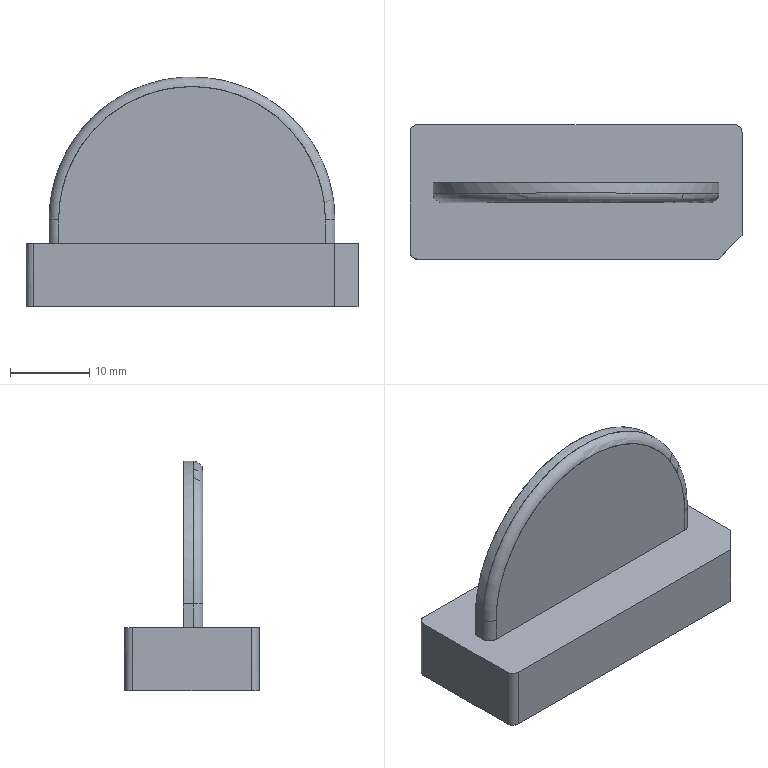NC program | PowerMill | posted with a generic post | part box 42 x 17 x 29.081 mm
Lines 5667 to 6702 of 145628:
N5764 M6
N5765 S18000 M03
N5766 G00 G90 X0.0 Y0.0
N5767 G43 Z9.788 H2
N5768
N5769 G05 P10000 R4
N5770 X-1.4388 Y4.1022
N5771 Z0.788
N5772 G01 Z-0.412 F3600.0
N5773 X-1.4486 Y4.0825 F6000.0
N5774 G03 X-1.3601 Y3.8169 I0.1771 J-0.0885
N5775 G01 X0.0 Y3.1368
N5776 X2.4403
N5777 X2.9283 Y3.1245
N5778 X3.4164 Y3.0087
N5779 X3.9826 Y2.6843
N5780 X4.4119 Y2.1962
N5781 X4.6322 Y1.7082
N5782 X4.7138 Y1.2201
N5783 X4.6788 Y0.4882
N5784 X4.6798 Y0.4753
N5785 X4.739 Y-0.244
N5786 X4.6595 Y-0.7321
N5787 X4.4429 Y-1.2201
N5788 X4.121 Y-1.7082
N5789 X3.9044 Y-1.9223
N5790 X3.4164 Y-2.2358
N5791 X2.4403 Y-2.5855
N5792 X1.9779 Y-2.6843
N5793 X1.4642 Y-2.7529
N5794 X0.4881 Y-2.8412
N5795 X-0.4881
N5796 X-1.9522 Y-2.6897
N5797 X-2.4403 Y-2.5855
N5798 X-3.4164 Y-2.2358
N5799 X-3.9044 Y-1.9215
N5800 X-4.121 Y-1.7082
N5801 X-4.4429 Y-1.2201
N5802 X-4.6589 Y-0.7321
N5803 X-4.7366 Y-0.244
N5804 X-4.6784 Y0.7321
N5805 X-4.6793 Y0.7453
N5806 X-4.715 Y1.2201
N5807 X-4.6322 Y1.7082
N5808 X-4.3925 Y2.2183
N5809 X-3.9837 Y2.6843
N5810 X-3.4164 Y3.0087
N5811 X-2.9283 Y3.1245
N5812 X-2.4403 Y3.1368
N5813 X0.0
N5814 X-1.4347 Y4.1022 Z-0.612
N5815 X-1.4446 Y4.0825
N5816 G03 X-1.3562 Y3.8169 I0.1771 J-0.0886
N5817 G01 X0.0 Y3.138
N5818 X1.2714 Y3.1368
N5819 X2.5428 Y3.1343
N5820 X3.9044 Y3.1337
N5821 X4.3925 Y3.0498
N5822 X4.8805 Y2.8251
N5823 X5.0794 Y2.6843
N5824 X5.3686 Y2.388
N5825 X5.506 Y2.1962
N5826 X5.7297 Y1.7082
N5827 X5.8082 Y1.2201
N5828 X5.8132 Y-0.244
N5829 X5.7359 Y-0.7321
N5830 X5.5415 Y-1.2201
N5831 X5.3686 Y-1.5237
N5832 X5.2321 Y-1.7082
N5833 X4.8805 Y-2.0296
N5834 X4.6466 Y-2.1962
N5835 X4.3925 Y-2.3401
N5836 X3.9044 Y-2.5526
N5837 X3.4994 Y-2.6843
N5838 X2.9283 Y-2.8349
N5839 X1.4642 Y-3.0204
N5840 X0.4881 Y-3.0644
N5841 X-0.4881
N5842 X-1.4642 Y-3.0204
N5843 X-2.9283 Y-2.8349
N5844 X-3.4164 Y-2.7105
N5845 X-3.9044 Y-2.5526
N5846 X-4.3925 Y-2.3401
N5847 X-4.6472 Y-2.1962
N5848 X-4.8805 Y-2.0296
N5849 X-5.2316 Y-1.7082
N5850 X-5.3686 Y-1.5237
N5851 X-5.5381 Y-1.2201
N5852 X-5.7396 Y-0.7321
N5853 X-5.8186 Y-0.244
N5854 X-5.8097 Y1.2201
N5855 X-5.7263 Y1.7082
N5856 X-5.5078 Y2.1962
N5857 X-5.3686 Y2.388
N5858 X-5.0772 Y2.6843
N5859 X-4.8805 Y2.8251
N5860 X-4.3925 Y3.0498
N5861 X-3.9044 Y3.1337
N5862 X-1.9522 Y3.1374
N5863 X0.0 Y3.138
N5864 X-1.4387 Y4.1021 Z-0.8119
N5865 X-1.4485 Y4.0825
N5866 G03 X-1.3599 Y3.8168 I0.1771 J-0.0886
N5867 G01 X0.0 Y3.1368
N5868 X4.3925
N5869 X4.8805 Y3.1211
N5870 X5.3686 Y2.9967
N5871 X5.8566 Y2.7189
N5872 X6.3328 Y2.1962
N5873 X6.5531 Y1.7082
N5874 X6.6352 Y1.2201
N5875 X6.621 Y0.4879
N5876 X6.6214 Y0.4803
N5877 Y0.4802
N5878 X6.6635 Y-0.244
N5879 X6.584 Y-0.7321
N5880 X6.4007 Y-1.2201
N5881 X6.0921 Y-1.7082
N5882 X5.8566 Y-1.9397
N5883 X5.3686 Y-2.3026
N5884 X4.5495 Y-2.6843
N5885 X3.9044 Y-2.8709
N5886 X2.9283 Y-3.0476
N5887 X1.6552 Y-3.1723
N5888 X0.4881 Y-3.2087
N5889 X-0.4881
N5890 X-1.6535 Y-3.1723
N5891 X-2.9283 Y-3.0476
N5892 X-3.9044 Y-2.8709
N5893 X-4.5513 Y-2.6843
N5894 X-5.3686 Y-2.3026
N5895 X-5.8566 Y-1.9397
N5896 X-6.088 Y-1.7082
N5897 X-6.3447 Y-1.3316
N5898 X-6.5833 Y-0.7321
N5899 X-6.6608 Y-0.244
N5900 X-6.6264 Y0.244
N5901 X-6.6342 Y1.2201
N5902 X-6.5531 Y1.7082
N5903 X-6.3338 Y2.1962
N5904 X-5.9035 Y2.6843
N5905 X-5.3686 Y2.9967
N5906 X-4.8805 Y3.1211
N5907 X-4.3925 Y3.1368
N5908 X0.0
N5909 X-1.4387 Y4.1022 Z-1.0119
N5910 X-1.4486 Y4.0825
N5911 G03 X-1.36 Y3.8168 I0.1771 J-0.0886
N5912 G01 X0.0 Y3.1368
N5913 X5.3686
N5914 X5.8566 Y3.0729
N5915 X6.3447 Y2.8729
N5916 X6.623 Y2.6843
N5917 X6.8327 Y2.4836
N5918 X7.0523 Y2.1962
N5919 X7.2726 Y1.7082
N5920 X7.3534 Y1.2201
N5921 X7.327 Y0.7321
N5922 X7.3498 Y-0.244
N5923 X7.2713 Y-0.7321
N5924 X7.0842 Y-1.2201
N5925 X6.8327 Y-1.6359
N5926 X6.3447 Y-2.1246
N5927 X5.8566 Y-2.4478
N5928 X5.3916 Y-2.6843
N5929 X4.3925 Y-2.9775
N5930 X3.9044 Y-3.0692
N5931 X3.1404 Y-3.1723
N5932 X1.4642 Y-3.2847
N5933 X-0.4881 Y-3.3013
N5934 X-1.9522 Y-3.2605
N5935 X-3.4164 Y-3.1416
N5936 X-4.3925 Y-2.9775
N5937 X-5.3917 Y-2.6843
N5938 X-5.8566 Y-2.4478
N5939 X-6.2581 Y-2.1962
N5940 X-6.7762 Y-1.7082
N5941 X-7.0853 Y-1.2201
N5942 X-7.272 Y-0.7321
N5943 X-7.3508 Y-0.244
N5944 X-7.3236 Y0.7321
N5945 X-7.3242 Y0.741
N5946 Y0.7411
N5947 X-7.3542 Y1.2201
N5948 X-7.2726 Y1.7082
N5949 X-7.0523 Y2.1962
N5950 X-6.8327 Y2.4836
N5951 X-6.623 Y2.6843
N5952 X-6.3447 Y2.8729
N5953 X-5.8566 Y3.0729
N5954 X-5.3686 Y3.1368
N5955 X0.0
N5956 X-1.4387 Y4.1022 Z-1.2119
N5957 X-1.4485 Y4.0825
N5958 G03 X-1.36 Y3.8168 I0.1771 J-0.0886
N5959 G01 X0.0 Y3.1368
N5960 X5.8566
N5961 X6.3447 Y3.0956
N5962 X6.8327 Y2.9254
N5963 X7.2075 Y2.6843
N5964 X7.3208 Y2.5827
N5965 X7.6368 Y2.1962
N5966 X7.8571 Y1.7082
N5967 X7.9383 Y1.2201
N5968 X7.9257 Y0.7321
N5969 X7.9494 Y-0.244
N5970 X7.8698 Y-0.7321
N5971 X7.703 Y-1.2201
N5972 X7.3929 Y-1.7082
N5973 X6.9164 Y-2.1962
N5974 X6.3447 Y-2.5496
N5975 X6.0719 Y-2.6843
N5976 X5.3686 Y-2.9288
N5977 X4.8805 Y-3.0476
N5978 X4.1428 Y-3.1723
N5979 X3.4164 Y-3.253
N5980 X1.4642 Y-3.3454
N5981 X-1.4642
N5982 X-2.9283 Y-3.289
N5983 X-4.3925 Y-3.1385
N5984 X-5.3686 Y-2.9288
N5985 X-5.8566 Y-2.7628
N5986 X-6.3447 Y-2.5496
N5987 X-6.8327 Y-2.2565
N5988 X-7.3208 Y-1.7872
N5989 X-7.703 Y-1.2201
N5990 X-7.8693 Y-0.7321
N5991 X-7.9487 Y-0.244
N5992 X-7.9242 Y0.244
N5993 X-7.9243 Y0.2504
N5994 Y0.2505
N5995 X-7.9387 Y1.2201
N5996 X-7.8571 Y1.7082
N5997 X-7.6368 Y2.1962
N5998 X-7.3208 Y2.5827
N5999 X-7.2074 Y2.6843
N6000 X-6.8327 Y2.9254
N6001 X-6.3447 Y3.0956
N6002 X-5.8566 Y3.1368
N6003 X0.0
N6004 X-1.4322 Y4.0989 Z-1.4119
N6005 X-1.4421 Y4.0792
N6006 G03 X-1.3535 Y3.8136 I0.1771 J-0.0885
N6007 G01 X0.0 Y3.1368
N6008 X6.3447
N6009 X6.8327 Y3.112
N6010 X7.3208 Y2.9687
N6011 X7.7903 Y2.6843
N6012 X8.2192 Y2.1962
N6013 X8.4394 Y1.7082
N6014 X8.5209 Y1.2201
N6015 X8.5323 Y-0.244
N6016 X8.4531 Y-0.7321
N6017 X8.2888 Y-1.2201
N6018 X7.9775 Y-1.7082
N6019 X7.5026 Y-2.1962
N6020 X6.8327 Y-2.6197
N6021 X6.3447 Y-2.829
N6022 X5.8566 Y-2.9875
N6023 X4.9753 Y-3.1723
N6024 X4.3925 Y-3.2512
N6025 X3.4164 Y-3.3261
N6026 X1.4642 Y-3.3698
N6027 X-2.9283 Y-3.3504
N6028 X-3.9044 Y-3.2945
N6029 X-4.8805 Y-3.1866
N6030 X-5.8566 Y-2.9875
N6031 X-6.3447 Y-2.829
N6032 X-6.8327 Y-2.6197
N6033 X-7.5028 Y-2.1962
N6034 X-7.9784 Y-1.7082
N6035 X-8.2888 Y-1.2201
N6036 X-8.4528 Y-0.7321
N6037 X-8.5318 Y-0.244
N6038 X-8.5198 Y1.2201
N6039 X-8.4395 Y1.7082
N6040 X-8.2198 Y2.1962
N6041 X-7.8088 Y2.6665
N6042 X-7.3208 Y2.9687
N6043 X-6.8327 Y3.112
N6044 X-6.3447 Y3.1368
N6045 X0.0
N6046 X-1.4388 Y4.1022 Z-1.6119
N6047 X-1.4486 Y4.0825
N6048 G03 X-1.3601 Y3.8169 I0.1771 J-0.0885
N6049 G01 X0.0 Y3.1368
N6050 X6.8327
N6051 X7.3208 Y3.108
N6052 X7.8088 Y2.9586
N6053 X8.2505 Y2.6843
N6054 X8.6798 Y2.1962
N6055 X8.9001 Y1.7082
N6056 X8.9817 Y1.2201
N6057 X8.9866 Y-0.244
N6058 X8.9081 Y-0.7321
N6059 X8.7849 Y-1.1407
N6060 X8.4477 Y-1.7082
N6061 X8.2969 Y-1.9007
N6062 X7.9954 Y-2.1962
N6063 X7.3208 Y-2.6438
N6064 X6.8327 Y-2.8483
N6065 X6.3447 Y-3.0055
N6066 X5.6236 Y-3.1723
N6067 X4.8805 Y-3.2782
N6068 X3.9044 Y-3.35
N6069 X2.4403 Y-3.3743
N6070 X-2.4403
N6071 X-3.9044 Y-3.35
N6072 X-4.8805 Y-3.2782
N6073 X-5.8566 Y-3.1337
N6074 X-6.8327 Y-2.8483
N6075 X-7.2321 Y-2.6843
N6076 X-7.9961 Y-2.1962
N6077 X-8.2969 Y-1.9007
N6078 X-8.4464 Y-1.7082
N6079 X-8.7542 Y-1.2201
N6080 X-8.9074 Y-0.7321
N6081 X-8.9866 Y-0.244
N6082 X-8.969 Y0.244
N6083 X-8.9691 Y0.2489
N6084 X-8.9811 Y1.2201
N6085 X-8.8999 Y1.7082
N6086 X-8.6801 Y2.1962
N6087 X-8.2969 Y2.6425
N6088 X-7.8088 Y2.9586
N6089 X-7.3208 Y3.108
N6090 X-6.8327 Y3.1368
N6091 X0.0
N6092 X-1.4379 Y4.1018 Z-1.8118
N6093 X-1.4478 Y4.0821
N6094 G03 X-1.3592 Y3.8164 I0.1771 J-0.0886
N6095 G01 X0.0 Y3.1368
N6096 X7.3208
N6097 X7.8088 Y3.1068
N6098 X8.2969 Y2.9549
N6099 X8.7278 Y2.6843
N6100 X9.1581 Y2.1962
N6101 X9.273 Y1.9837
N6102 X9.3772 Y1.7082
N6103 X9.4616 Y1.2201
N6104 X9.4393 Y0.7321
N6105 X9.4395 Y0.7254
N6106 X9.4598 Y-0.244
N6107 X9.3817 Y-0.7321
N6108 X9.2259 Y-1.2201
N6109 X8.9205 Y-1.7082
N6110 X8.7849 Y-1.882
N6111 X8.4693 Y-2.1962
N6112 X7.8088 Y-2.6394
N6113 X7.3208 Y-2.8668
N6114 X6.8327 Y-3.0253
N6115 X6.2056 Y-3.1723
N6116 X5.8566 Y-3.2351
N6117 X4.8805 Y-3.3365
N6118 X3.4164 Y-3.3743
N6119 X-3.4164
N6120 X-4.3925 Y-3.3583
N6121 X-5.3686 Y-3.2947
N6122 X-6.3447 Y-3.1474
N6123 X-6.8327 Y-3.0253
N6124 X-7.3208 Y-2.8668
N6125 X-7.8088 Y-2.6394
N6126 X-8.4695 Y-2.1962
N6127 X-8.7849 Y-1.882
N6128 X-8.9205 Y-1.7082
N6129 X-9.2275 Y-1.2201
N6130 X-9.3815 Y-0.7321
N6131 X-9.4596 Y-0.244
N6132 X-9.4376 Y0.244
N6133 X-9.4377 Y0.2508
N6134 X-9.4604 Y1.2201
N6135 X-9.3805 Y1.7082
N6136 X-9.273 Y1.9837
N6137 X-9.1595 Y2.1962
N6138 X-8.7849 Y2.6373
N6139 X-8.2969 Y2.9549
N6140 X-7.8088 Y3.1068
N6141 X-7.3208 Y3.1368
N6142 X0.0
N6143 X-1.4388 Y4.1022 Z-2.0118
N6144 X-1.4486 Y4.0825
N6145 G03 X-1.3601 Y3.8169 I0.1771 J-0.0885
N6146 G01 X0.0 Y3.1368
N6147 X7.8088
N6148 X8.2969 Y3.0927
N6149 X8.7849 Y2.9188
N6150 X9.1462 Y2.6843
N6151 X9.273 Y2.5695
N6152 X9.5749 Y2.1962
N6153 X9.7611 Y1.8093
N6154 X9.877 Y1.2201
N6155 X9.8838 Y-0.244
N6156 X9.8046 Y-0.7321
N6157 X9.6484 Y-1.2201
N6158 X9.273 Y-1.8214
N6159 X8.9112 Y-2.1962
N6160 X8.2969 Y-2.6316
N6161 X7.8088 Y-2.8608
N6162 X7.3208 Y-3.0265
N6163 X6.7572 Y-3.1723
N6164 X6.3447 Y-3.2481
N6165 X5.3686 Y-3.3501
N6166 X4.3925 Y-3.3743
N6167 X-4.3925
N6168 X-5.3686 Y-3.3501
N6169 X-6.3447 Y-3.2481
N6170 X-6.8327 Y-3.1568
N6171 X-7.3208 Y-3.0265
N6172 X-7.8088 Y-2.8608
N6173 X-8.2969 Y-2.6316
N6174 X-8.7849 Y-2.2993
N6175 X-9.273 Y-1.8214
N6176 X-9.6484 Y-1.2201
N6177 X-9.7611 Y-0.8963
N6178 X-9.8835 Y-0.244
N6179 X-9.8773 Y1.2201
N6180 X-9.7954 Y1.7082
N6181 X-9.5755 Y2.1962
N6182 X-9.273 Y2.5695
N6183 X-9.1456 Y2.6843
N6184 X-8.7849 Y2.9188
N6185 X-8.2969 Y3.0927
N6186 X-7.8088 Y3.1368
N6187 X0.0
N6188 X-1.4388 Y4.1022 Z-2.2118
N6189 X-1.4487 Y4.0825
N6190 G03 X-1.3601 Y3.8168 I0.1771 J-0.0886
N6191 G01 X0.0 Y3.1368
N6192 X7.8088
N6193 X7.8099 Y3.1367
N6194 X7.815
N6195 X8.2969
N6196 X8.7849 Y3.0708
N6197 X9.273 Y2.8699
N6198 X9.5442 Y2.6843
N6199 X9.7611 Y2.4757
N6200 X9.9738 Y2.1962
N6201 X10.1939 Y1.7082
N6202 X10.275 Y1.2201
N6203 X10.2597 Y0.7321
N6204 X10.2831 Y-0.244
N6205 X10.2491 Y-0.5363
N6206 X10.0552 Y-1.2201
N6207 X9.7574 Y-1.7082
N6208 X9.3169 Y-2.1962
N6209 X8.7849 Y-2.5911
N6210 X8.2969 Y-2.8457
N6211 X7.8088 Y-3.0217
N6212 X7.2298 Y-3.1723
N6213 X6.8327 Y-3.2535
N6214 X5.8566 Y-3.3524
N6215 X4.8805 Y-3.3743
N6216 X-4.8805
N6217 X-5.8566 Y-3.3524
N6218 X-6.8327 Y-3.2535
N6219 X-7.3208 Y-3.1532
N6220 X-7.8088 Y-3.0217
N6221 X-8.2969 Y-2.8457
N6222 X-8.7849 Y-2.5911
N6223 X-9.273 Y-2.2333
N6224 X-9.7611 Y-1.706
N6225 X-10.0552 Y-1.2201
N6226 X-10.2069 Y-0.7321
N6227 X-10.2817 Y-0.244
N6228 X-10.2601 Y0.244
N6229 X-10.2752 Y1.2201
N6230 X-10.1936 Y1.7082
N6231 X-9.973 Y2.1962
N6232 X-9.7611 Y2.4757
N6233 X-9.5442 Y2.6843
N6234 X-9.273 Y2.8699
N6235 X-8.7849 Y3.0708
N6236 X-8.2969 Y3.1367
N6237 X-7.8099
N6238 X-7.8088 Y3.1368
N6239 X0.0
N6240 X-1.4387 Y4.1022 Z-2.4118
N6241 X-1.4486 Y4.0825
N6242 G03 X-1.36 Y3.8168 I0.1771 J-0.0886
N6243 G01 X0.0 Y3.1368
N6244 X8.2969
N6245 X8.7849 Y3.1322
N6246 X9.273 Y3.0393
N6247 X9.7611 Y2.8033
N6248 X9.924 Y2.6843
N6249 X10.2491 Y2.346
N6250 X10.3538 Y2.1962
N6251 X10.5735 Y1.7082
N6252 X10.6553 Y1.2201
N6253 X10.6409 Y0.7321
N6254 X10.641 Y0.7273
N6255 X10.6592 Y-0.244
N6256 X10.5843 Y-0.7321
N6257 X10.4349 Y-1.2201
N6258 X10.154 Y-1.7082
N6259 X9.7611 Y-2.1596
N6260 X9.273 Y-2.5425
N6261 X8.7849 Y-2.8077
N6262 X8.2969 Y-3.0005
N6263 X7.7024 Y-3.1723
N6264 X7.3208 Y-3.2503
N6265 X6.3447 Y-3.3542
N6266 X5.3686 Y-3.3743
N6267 X-4.8805
N6268 X-6.3447 Y-3.3542
N6269 X-7.3208 Y-3.2503
N6270 X-7.8088 Y-3.1472
N6271 X-8.2969 Y-3.0005
N6272 X-8.7849 Y-2.8077
N6273 X-9.273 Y-2.5425
N6274 X-9.7212 Y-2.1962
N6275 X-10.1532 Y-1.7082
N6276 X-10.4344 Y-1.2201
N6277 X-10.5865 Y-0.7321
N6278 X-10.6595 Y-0.244
N6279 X-10.6411 Y0.244
N6280 X-10.6412 Y0.2493
N6281 X-10.6555 Y1.2201
N6282 X-10.5729 Y1.7082
N6283 X-10.3533 Y2.1962
N6284 X-10.2491 Y2.346
N6285 X-9.9239 Y2.6843
N6286 X-9.7611 Y2.8033
N6287 X-9.273 Y3.0393
N6288 X-8.7849 Y3.1322
N6289 X-8.2969 Y3.1368
N6290 X0.0
N6291 X-1.4365 Y4.1011 Z-2.6118
N6292 X-1.4463 Y4.0814
N6293 G03 X-1.3578 Y3.8157 I0.177 J-0.0886
N6294 G01 X0.0 Y3.1368
N6295 X8.7849
N6296 X9.273 Y3.12
N6297 X9.7611 Y2.9946
N6298 X10.2491 Y2.7158
N6299 X10.7185 Y2.1962
N6300 X10.9382 Y1.7082
N6301 X11.0204 Y1.2201
N6302 X11.0217 Y-0.244
N6303 X10.941 Y-0.7321
N6304 X10.789 Y-1.2201
N6305 X10.5076 Y-1.7082
N6306 X10.2491 Y-2.0305
N6307 X9.7611 Y-2.4647
N6308 X9.273 Y-2.764
N6309 X8.7849 Y-2.9711
N6310 X8.1085 Y-3.1723
N6311 X7.8088 Y-3.2419
N6312 X7.3208 Y-3.3104
N6313 X6.3447 Y-3.3718
N6314 X5.4897
N6315 X5.3686 Y-3.3743
N6316 X-4.8805
N6317 X-5.0623 Y-3.3718
N6318 X-5.0636
N6319 X-6.3447
N6320 X-6.8327 Y-3.3537
N6321 X-7.8088 Y-3.2419
N6322 X-8.2969 Y-3.1277
N6323 X-8.7849 Y-2.9711
N6324 X-9.273 Y-2.764
N6325 X-9.7611 Y-2.4647
N6326 X-10.2491 Y-2.0305
N6327 X-10.5076 Y-1.7082
N6328 X-10.7886 Y-1.2201
N6329 X-10.9399 Y-0.7321
N6330 X-11.0198 Y-0.244
N6331 X-11.0202 Y1.2201
N6332 X-10.9388 Y1.7082
N6333 X-10.7372 Y2.1637
N6334 X-10.2893 Y2.6843
N6335 X-9.7611 Y2.9946
N6336 X-9.273 Y3.12
N6337 X-8.7849 Y3.1368
N6338 X0.0
N6339 X-1.4387 Y4.1022 Z-2.8117
N6340 X-1.4485 Y4.0825
N6341 G03 X-1.3599 Y3.8169 I0.1771 J-0.0886
N6342 G01 X0.0 Y3.1369
N6343 X9.273
N6344 X9.7611 Y3.0937
N6345 X10.2491 Y2.924
N6346 X10.6197 Y2.6843
N6347 X10.7372 Y2.5784
N6348 X11.0487 Y2.1962
N6349 X11.2691 Y1.7082
N6350 X11.3504 Y1.2201
N6351 X11.3593 Y-0.244
N6352 X11.2901 Y-0.7321
N6353 X11.1431 Y-1.2201
N6354 X10.7372 Y-1.8819
N6355 X10.2491 Y-2.3602
N6356 X9.7611 Y-2.6847
N6357 X9.273 Y-2.9251
N6358 X8.7849 Y-3.1046
N6359 X8.5143 Y-3.1723
N6360 X8.2969 Y-3.2239
N6361 X7.3208 Y-3.3524
N6362 X6.3447 Y-3.3743
N6363 X-5.3686
N6364 X-6.0189 Y-3.3741
N6365 X-6.6691 Y-3.3597
N6366 X-6.6716
N6367 X-7.3208 Y-3.3524
N6368 X-8.2969 Y-3.2239
N6369 X-8.7849 Y-3.1046
N6370 X-9.273 Y-2.9251
N6371 X-9.7611 Y-2.6843
N6372 X-10.2491 Y-2.3602
N6373 X-10.7372 Y-1.8819
N6374 X-10.8619 Y-1.7082
N6375 X-11.1427 Y-1.2201
N6376 X-11.2911 Y-0.7321
N6377 X-11.3595 Y-0.244
N6378 X-11.3413 Y0.244
N6379 X-11.3506 Y1.2201
N6380 X-11.2693 Y1.7082
N6381 X-11.0492 Y2.1962
N6382 X-10.7372 Y2.5784
N6383 X-10.6199 Y2.6843
N6384 X-10.2491 Y2.924
N6385 X-9.7611 Y3.0937
N6386 X-9.273 Y3.1369
N6387 X0.0
N6388 X-1.4311 Y4.0983 Z-3.0117
N6389 X-1.4409 Y4.0787
N6390 G03 X-1.3524 Y3.813 I0.1771 J-0.0886
N6391 G01 X0.0 Y3.1368
N6392 X9.273
N6393 X9.3064 Y3.1339
N6394 X9.7611 Y3.1338
N6395 X10.2491 Y3.0526
N6396 X10.7372 Y2.8308
N6397 X10.9426 Y2.6843
N6398 X11.2252 Y2.3996
N6399 X11.372 Y2.1962
N6400 X11.5922 Y1.7082
N6401 X11.6738 Y1.2201
N6402 X11.6575 Y0.7321
N6403 X11.6705 Y-0.244
N6404 X11.6025 Y-0.7321
N6405 X11.4548 Y-1.2201
N6406 X11.2252 Y-1.6449
N6407 X10.7666 Y-2.1962
N6408 X10.2491 Y-2.6036
N6409 X9.7611 Y-2.871
N6410 X9.273 Y-3.064
N6411 X8.8835 Y-3.1723
N6412 X8.2969 Y-3.2896
N6413 X7.8088 Y-3.3479
N6414 X6.8327 Y-3.3743
N6415 X-6.3447
N6416 X-7.8088 Y-3.3479
N6417 X-8.2969 Y-3.2896
N6418 X-8.7849 Y-3.1982
N6419 X-9.273 Y-3.064
N6420 X-9.7611 Y-2.871
N6421 X-10.1159 Y-2.6843
N6422 X-10.7372 Y-2.2261
N6423 X-11.1871 Y-1.7082
N6424 X-11.4551 Y-1.2201
N6425 X-11.6019 Y-0.7321
N6426 X-11.6707 Y-0.244
N6427 X-11.6574 Y0.244
N6428 Y0.2484
N6429 X-11.6739 Y1.2201
N6430 X-11.5909 Y1.7082
N6431 X-11.3703 Y2.1962
N6432 X-11.2252 Y2.3996
N6433 X-10.9422 Y2.6843
N6434 X-10.7372 Y2.8308
N6435 X-10.2491 Y3.0526
N6436 X-9.7611 Y3.1338
N6437 X-9.273 Y3.1369
N6438 X-8.9563 Y3.1368
N6439 X0.0
N6440 X-1.4386 Y4.1021 Z-3.2117
N6441 X-1.4485 Y4.0825
N6442 G03 X-1.3599 Y3.8168 I0.1771 J-0.0886
N6443 G01 X0.0 Y3.1369
N6444 X9.7611
N6445 X10.2491 Y3.1179
N6446 X10.7372 Y2.9848
N6447 X11.2252 Y2.6983
N6448 X11.6725 Y2.1962
N6449 X11.8926 Y1.7082
N6450 X11.9743 Y1.2201
N6451 X11.9818 Y-0.244
N6452 X11.9136 Y-0.7321
N6453 X11.7661 Y-1.2201
N6454 X11.4983 Y-1.7082
N6455 X11.2252 Y-2.0467
N6456 X10.7372 Y-2.4887
N6457 X10.2491 Y-2.7964
N6458 X9.7611 Y-3.0141
N6459 X9.2374 Y-3.1723
N6460 X8.7849 Y-3.2702
N6461 X8.2969 Y-3.3401
N6462 X7.3208 Y-3.3743
N6463 X-7.3208
N6464 X-8.2969 Y-3.3401
N6465 X-8.7849 Y-3.2702
N6466 X-9.2368 Y-3.1723
N6467 X-9.7611 Y-3.0141
N6468 X-10.2491 Y-2.7964
N6469 X-10.7372 Y-2.4887
N6470 X-11.0765 Y-2.1962
N6471 X-11.4983 Y-1.7082
N6472 X-11.7661 Y-1.2201
N6473 X-11.9127 Y-0.7321
N6474 X-11.9819 Y-0.244
N6475 X-11.9746 Y1.2201
N6476 X-11.8929 Y1.7082
N6477 X-11.7133 Y2.1261
N6478 X-11.2431 Y2.6843
N6479 X-10.7372 Y2.9848
N6480 X-10.2491 Y3.1179
N6481 X-9.7611 Y3.1369
N6482 X0.0
N6483 X-1.4386 Y4.1021 Z-3.4117
N6484 X-1.4485 Y4.0825
N6485 G03 X-1.3599 Y3.8168 I0.1771 J-0.0886
N6486 G01 X0.0 Y3.1369
N6487 X10.2491
N6488 X10.7372 Y3.0853
N6489 X11.2252 Y2.9031
N6490 X11.5544 Y2.6843
N6491 X11.7133 Y2.5388
N6492 X11.9836 Y2.1962
N6493 X12.2039 Y1.7082
N6494 X12.2856 Y1.2201
N6495 X12.2863 Y-0.244
N6496 X12.2177 Y-0.7321
N6497 X12.0708 Y-1.2201
N6498 X11.8095 Y-1.7082
N6499 X11.7133 Y-1.8432
N6500 X11.2252 Y-2.3519
N6501 X10.7372 Y-2.6946
N6502 X10.2491 Y-2.9398
N6503 X9.5826 Y-3.1723
N6504 X9.273 Y-3.25
N6505 X8.7849 Y-3.3233
N6506 X7.8088 Y-3.3743
N6507 X-7.8088
N6508 X-8.7849 Y-3.3233
N6509 X-9.273 Y-3.25
N6510 X-9.5819 Y-3.1723
N6511 X-10.2491 Y-2.9398
N6512 X-10.7516 Y-2.6843
N6513 X-11.2252 Y-2.3519
N6514 X-11.7133 Y-1.8432
N6515 X-11.8095 Y-1.7082
N6516 X-12.0708 Y-1.2201
N6517 X-12.2013 Y-0.8163
N6518 X-12.2859 Y-0.244
N6519 X-12.2854 Y1.2201
N6520 X-12.2013 Y1.7125
N6521 X-11.9837 Y2.1962
N6522 X-11.7133 Y2.5388
N6523 X-11.5544 Y2.6843
N6524 X-11.2252 Y2.9031
N6525 X-10.7372 Y3.0853
N6526 X-10.2491 Y3.1369
N6527 X0.0
N6528 X-1.4347 Y4.1002 Z-3.6117
N6529 X-1.4445 Y4.0805
N6530 G03 X-1.356 Y3.8149 I0.1771 J-0.0885
N6531 G01 X0.0 Y3.1369
N6532 X10.2491
N6533 X10.7372 Y3.1295
N6534 X11.2252 Y3.0249
N6535 X11.7133 Y2.7752
N6536 X11.8349 Y2.6843
N6537 X12.2642 Y2.1962
N6538 X12.4844 Y1.7082
N6539 X12.566 Y1.2201
N6540 X12.5603 Y-0.244
N6541 X12.4929 Y-0.7321
N6542 X12.346 Y-1.2201
N6543 X12.0879 Y-1.7082
N6544 X11.6823 Y-2.1962
N6545 X11.2252 Y-2.5739
N6546 X10.7372 Y-2.8611
N6547 X10.2491 Y-3.0665
N6548 X9.8937 Y-3.1723
N6549 X9.273 Y-3.3009
N6550 X8.7849 Y-3.3547
N6551 X8.2969 Y-3.3743
N6552 X-8.2969
N6553 X-8.7849 Y-3.3547
N6554 X-9.273 Y-3.3009
N6555 X-9.7611 Y-3.2105
N6556 X-10.2491 Y-3.0665
N6557 X-10.7372 Y-2.8611
N6558 X-11.0631 Y-2.6843
N6559 X-11.6816 Y-2.1962
N6560 X-12.087 Y-1.7082
N6561 X-12.346 Y-1.2201
N6562 X-12.4931 Y-0.7321
N6563 X-12.56 Y-0.244
N6564 X-12.566 Y1.2201
N6565 X-12.484 Y1.7082
N6566 X-12.2639 Y2.1962
N6567 X-11.8349 Y2.6843
N6568 X-11.7133 Y2.7752
N6569 X-11.2252 Y3.0249
N6570 X-10.7372 Y3.1295
N6571 X-10.2491 Y3.1369
N6572 X0.0
N6573 X-1.4387 Y4.1022 Z-3.8117
N6574 X-1.4485 Y4.0825
N6575 G03 X-1.36 Y3.8169 I0.1771 J-0.0885
N6576 G01 X0.0 Y3.1369
N6577 X10.7372
N6578 X11.2252 Y3.0966
N6579 X11.7133 Y2.93
N6580 X12.0963 Y2.6843
N6581 X12.2013 Y2.5896
N6582 X12.5256 Y2.1962
N6583 X12.6894 Y1.8702
N6584 X12.7459 Y1.7082
N6585 X12.8275 Y1.2201
N6586 X12.8343 Y-0.244
N6587 X12.7681 Y-0.7321
N6588 X12.6213 Y-1.2201
N6589 X12.3628 Y-1.7082
N6590 X11.9571 Y-2.1962
N6591 X11.7133 Y-2.4188
N6592 X11.3447 Y-2.6843
N6593 X10.7372 Y-2.9981
N6594 X10.2047 Y-3.1723
N6595 X9.7611 Y-3.2726
N6596 X9.273 Y-3.3439
N6597 X8.2969 Y-3.3743
N6598 X8.0006
N6599 X-8.2969
N6600 X-8.3672 Y-3.3714
N6601 X-8.3712
N6602 X-8.7849
N6603 X-9.273 Y-3.3439
N6604 X-9.7611 Y-3.2726
N6605 X-10.2051 Y-3.1723
N6606 X-10.7372 Y-2.9981
N6607 X-11.2252 Y-2.7575
N6608 X-11.7133 Y-2.4188
N6609 X-11.9572 Y-2.1962
N6610 X-12.3628 Y-1.7082
N6611 X-12.6213 Y-1.2201
N6612 X-12.7683 Y-0.7321
N6613 X-12.8342 Y-0.244
N6614 X-12.8274 Y1.2201
N6615 X-12.7455 Y1.7082
N6616 X-12.6894 Y1.8702
N6617 X-12.5254 Y2.1962
N6618 X-12.2013 Y2.5896
N6619 X-12.0962 Y2.6843
N6620 X-11.7133 Y2.93
N6621 X-11.2252 Y3.0966
N6622 X-10.7372 Y3.1369
N6623 X0.0
N6624 X-1.4387 Y4.1022 Z-4.0116
N6625 X-1.4485 Y4.0825
N6626 G03 X-1.36 Y3.8169 I0.1771 J-0.0885
N6627 G01 X0.0 Y3.1369
N6628 X10.7372
N6629 X11.2252 Y3.1315
N6630 X11.7133 Y3.0364
N6631 X12.2013 Y2.7995
N6632 X12.3577 Y2.6843
N6633 X12.6894 Y2.3369
N6634 X12.7871 Y2.1962
N6635 X13.0074 Y1.7082
N6636 X13.089 Y1.2201
N6637 X13.1019 Y-0.244
N6638 X13.0386 Y-0.7321
N6639 X12.8916 Y-1.2201
N6640 X12.6894 Y-1.6203
N6641 X12.232 Y-2.1962
N6642 X11.7133 Y-2.6187
N6643 X11.2252 Y-2.8966
N6644 X10.502 Y-3.1723
N6645 X10.2491 Y-3.2404
N6646 X9.7611 Y-3.3229
N6647 X8.7849 Y-3.3743
N6648 X-8.7849
N6649 X-9.7611 Y-3.3229
N6650 X-10.2491 Y-3.2404
N6651 X-10.5016 Y-3.1723
N6652 X-11.2252 Y-2.8966
N6653 X-11.6206 Y-2.6843
N6654 X-12.2013 Y-2.2288
N6655 X-12.6385 Y-1.7082
N6656 X-12.8917 Y-1.2201
N6657 X-13.0389 Y-0.7321
N6658 X-13.1023 Y-0.244
N6659 X-13.0888 Y1.2201
N6660 X-13.0071 Y1.7082
N6661 X-12.7869 Y2.1962
N6662 X-12.6894 Y2.3369
N6663 X-12.3576 Y2.6843
N6664 X-12.2013 Y2.7995
N6665 X-11.7133 Y3.0364
N6666 X-11.2252 Y3.1315
N6667 X-10.7372 Y3.1369
N6668 X0.0
N6669 X-1.4354 Y4.1005 Z-4.2116
N6670 X-1.4452 Y4.0808
N6671 G03 X-1.3566 Y3.8152 I0.1771 J-0.0885
N6672 G01 X0.0 Y3.1369
N6673 X11.2252
N6674 X11.7133 Y3.1025
N6675 X12.2013 Y2.9461
N6676 X12.6191 Y2.6843
N6677 X13.0485 Y2.1962
N6678 X13.1774 Y1.9499
N6679 X13.2689 Y1.7082
N6680 X13.3504 Y1.2201
N6681 X13.3542 Y-0.244
N6682 X13.2833 Y-0.7321
N6683 X13.1774 Y-1.1156
N6684 X12.8865 Y-1.7082
N6685 X12.4947 Y-2.1962
N6686 X12.2013 Y-2.4577
N6687 X11.8935 Y-2.6843
N6688 X11.2252 Y-3.0244
N6689 X10.7771 Y-3.1723
N6690 X10.2491 Y-3.2905
N6691 X9.7611 Y-3.3529
N6692 X9.273 Y-3.3743
N6693 X-9.273
N6694 X-9.7611 Y-3.3529
N6695 X-10.2491 Y-3.2905
N6696 X-10.7372 Y-3.1843
N6697 X-11.2252 Y-3.0244
N6698 X-11.7133 Y-2.791
N6699 X-12.2013 Y-2.4577
N6700 X-12.4944 Y-2.1962
N6701 X-12.8866 Y-1.7082
N6702 X-13.1362 Y-1.2201
N6703 X-13.2834 Y-0.7321
N6704 X-13.3545 Y-0.244
N6705 X-13.3506 Y1.2201
N6706 X-13.2683 Y1.7082
N6707 X-13.1774 Y1.9499
N6708 X-13.0487 Y2.1962
N6709 X-12.6894 Y2.6225
N6710 X-12.2013 Y2.9461
N6711 X-11.7133 Y3.1025
N6712 X-11.2252 Y3.1369
N6713 X0.0
N6714 X-1.4385 Y4.1021 Z-4.4116
N6715 X-1.4484 Y4.0824
N6716 G03 X-1.3598 Y3.8168 I0.1771 J-0.0885
N6717 G01 X0.0 Y3.1369
N6718 X11.2252
N6719 X11.7133 Y3.1322
N6720 X12.2013 Y3.0415
N6721 X12.6894 Y2.8088
N6722 X12.8604 Y2.6843
N6723 X13.1774 Y2.3564
N6724 X13.2896 Y2.1962
N6725 X13.5099 Y1.7082
N6726 X13.5915 Y1.2201
N6727 X13.597 Y-0.244
N6728 X13.5279 Y-0.7321
N6729 X13.3797 Y-1.2201
N6730 X13.1774 Y-1.6286
N6731 X12.7392 Y-2.1962
N6732 X12.2013 Y-2.6449
N6733 X11.7133 Y-2.9219
N6734 X11.0521 Y-3.1723
N6735 X10.2491 Y-3.3367
N6736 X9.273 Y-3.3743
N6737 X-9.273
N6738 X-10.2491 Y-3.3367
N6739 X-11.052 Y-3.1723
N6740 X-11.7133 Y-2.9219
N6741 X-12.1441 Y-2.6843
N6742 X-12.6894 Y-2.2471
N6743 X-13.1312 Y-1.7082
N6744 X-13.3808 Y-1.2201
N6745 X-13.5279 Y-0.7321
N6746 X-13.5968 Y-0.244
N6747 X-13.5915 Y1.2201
N6748 X-13.5099 Y1.7082
N6749 X-13.2896 Y2.1962
N6750 X-13.1774 Y2.3564
N6751 X-12.8603 Y2.6843
N6752 X-12.6894 Y2.8088
N6753 X-12.2013 Y3.0415
N6754 X-11.7133 Y3.1322
N6755 X-11.2252 Y3.1369
N6756 X0.0
N6757 X-1.4385 Y4.1021 Z-4.6116
N6758 X-1.4484 Y4.0824
N6759 G03 X-1.3598 Y3.8168 I0.1771 J-0.0885
N6760 G01 X0.0 Y3.1369
N6761 X11.7133
N6762 X12.2013 Y3.1004
N6763 X12.6894 Y2.9375
N6764 X13.1774 Y2.6063
N6765 X13.518 Y2.1962
N6766 X13.6655 Y1.9091
N6767 X13.7383 Y1.7082
N6768 X13.8199 Y1.2201
N6769 X13.8346 Y-0.244
N6770 X13.7725 Y-0.7321
N6771 X13.6655 Y-1.1198
N6772 X13.3755 Y-1.7082
N6773 X12.9837 Y-2.1962
N6774 X12.6894 Y-2.4585
N6775 X12.3888 Y-2.6843
N6776 X11.7133 Y-3.0346
N6777 X11.3157 Y-3.1723
N6778 X10.7372 Y-3.3018
N6779 X10.2491 Y-3.3564
N6780 X9.7611 Y-3.3743
N6781 X-9.7611
N6782 X-10.2491 Y-3.3564
N6783 X-10.7372 Y-3.3018
N6784 X-11.2252 Y-3.2009
N6785 X-11.7133 Y-3.0346
N6786 X-12.3891 Y-2.6843
N6787 X-12.6894 Y-2.4585
N6788 X-12.9836 Y-2.1962
N6789 X-13.3758 Y-1.7082
N6790 X-13.6254 Y-1.2201
N6791 X-13.7723 Y-0.7321
N6792 X-13.8344 Y-0.244
N6793 X-13.8199 Y1.2201
N6794 X-13.7383 Y1.7082
N6795 X-13.6655 Y1.9091
N6796 X-13.518 Y2.1962
N6797 X-13.1774 Y2.6063
N6798 X-12.6894 Y2.9375
N6799 X-12.2013 Y3.1004